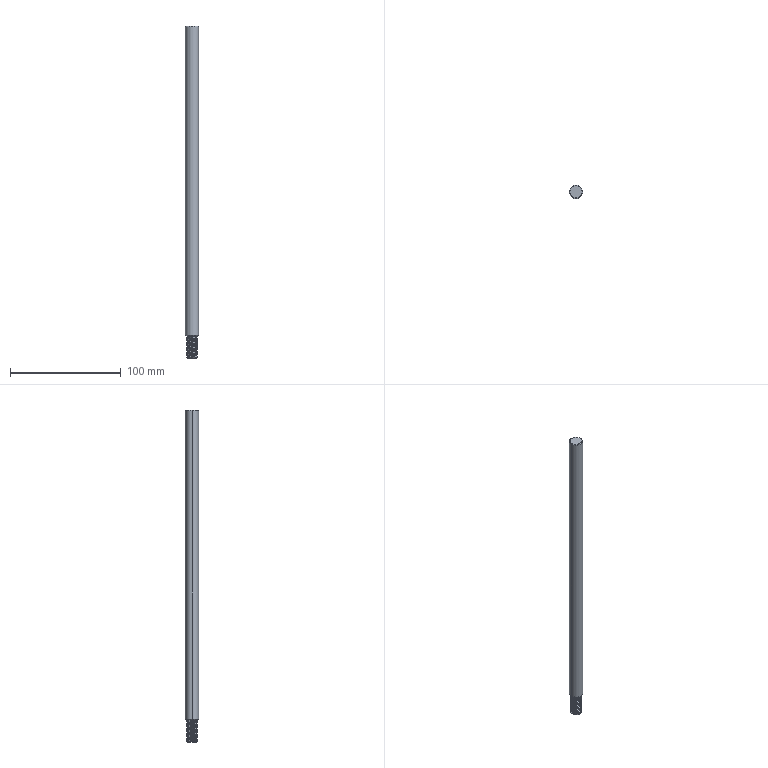Part | SolidWorks | features Chamfer 1, Extrusion 1, ICE 1, SweepThread 1 | 1 solid | 42 faces | box 12 x 12 x 300 mm | volume 32966 mm3 | cylinder 29 | cone 6 | plane 4 | spline 3 | commonest cylinder face diameters 10 x27 12 x2